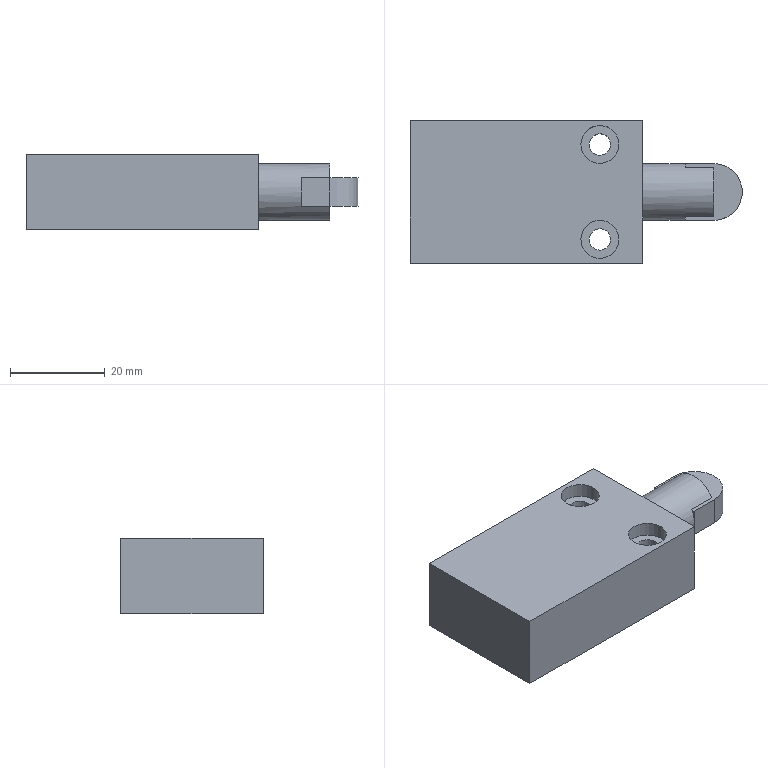Part | STEP file | solid 61 | 1 solid | 28 faces | box 70 x 30 x 16 mm | volume 24653 mm3 | plane 20 | cylinder 8 | commonest cylinder face diameters 8 x4 4.5 x2 12 x2